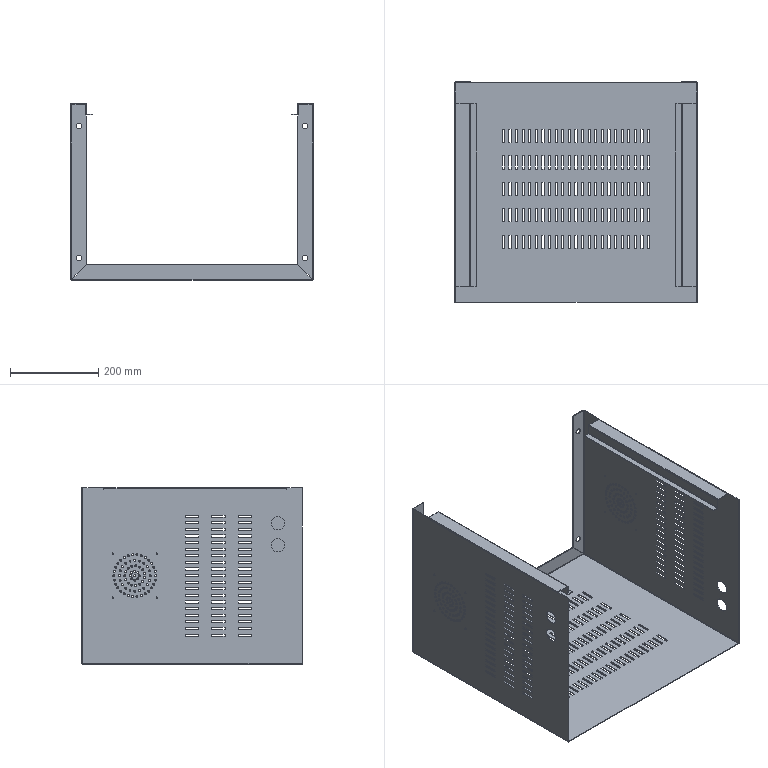Part | SolidWorks | features ICE 6, EdgeFlange 5, LPattern 3, FlatPattern 1, SMBaseFlange 1, SheetMetal 1 | 1 solid | 1354 faces | box 550 x 500 x 400 mm | volume 1097437 mm3 | plane 1000 | cylinder 350 | spline 4 | commonest cylinder face diameters 4.5 x296 3.2 x16 1 x11 4 x11 13 x8 30 x8